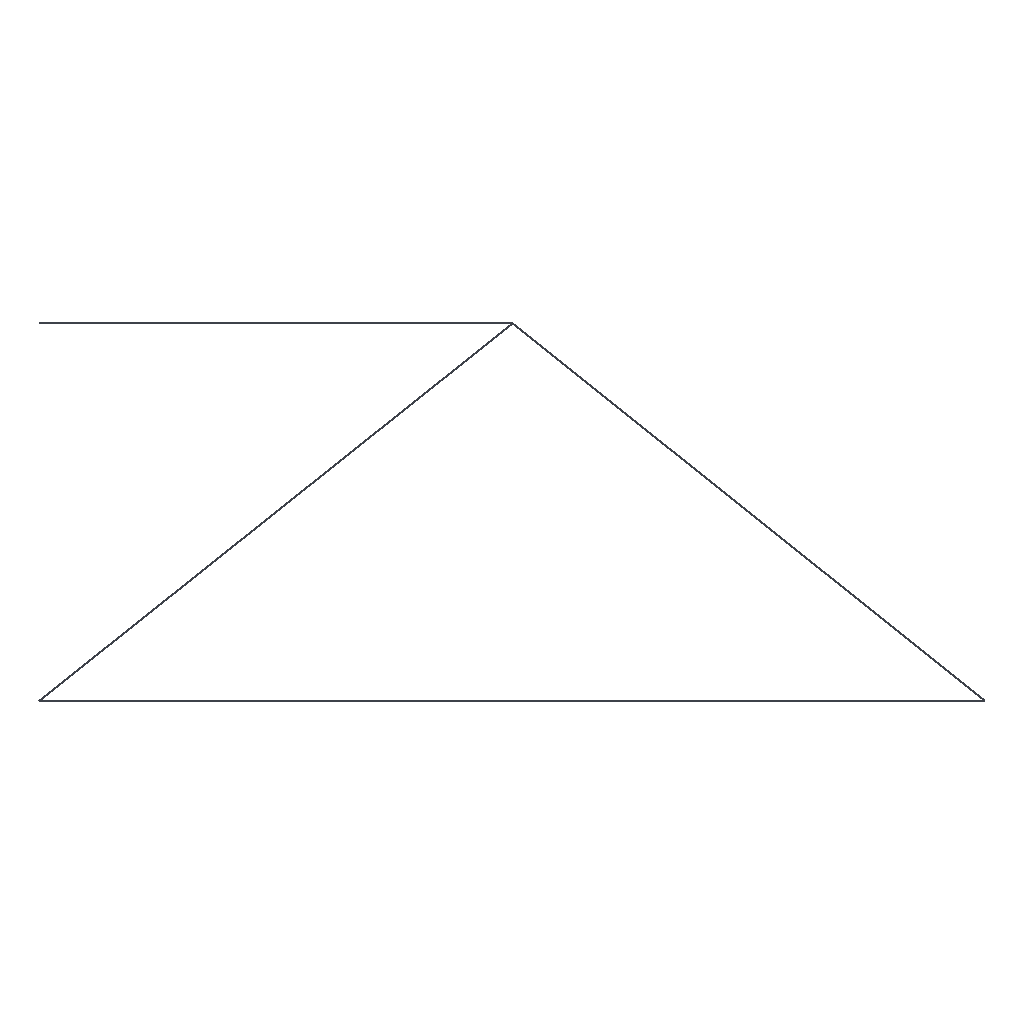Simulation study | abaqus
Set-up summary:
category,name,step,type,value,unit,region
solver,abaqus,,Abaqus/CAE 2024
units,mm-N-s-tonne (MPa),,inferred,E=295000 density=
analysis,Step-1,,static,time_period=1
mesh,nodes,,,4
mesh,elements,,,4
element_type,T2D2,,,4
material,Material-1,,E,295000
material,Material-1,,nu,0
section,Material-1,,solid section,,,_PickedSet2
load,Load-1,Step-1,concentrated force,"100 [dir=(0, -1, 0)]",,_PickedSet6
bc,BC-1,Step-1,fixed,"[dofs=x,y n=2]",,_PickedSet4
bc,BC-2,Step-1,fixed,[dofs=y],,_PickedSet5
Abaqus input file, long lists of numbers shortened:
*Heading
** Job name: deck Model name: link
** Generated by: Abaqus/CAE 2024
*Preprint, echo=NO, model=NO, history=NO, contact=NO
**
** PARTS
**
*Part, name=Part-1
*Node
      1,         100.,          80.
      2,           0.,          80.
** (2 more lines like these left out)
*Element, type=T2D2
1, 1, 2
2, 3, 1
** (2 more lines like these left out)
*Nset, nset=_PickedSet2, internal, generate
 1,  4,  1
*Elset, elset=_PickedSet2, internal, generate
 1,  4,  1
** Section: Section-1
*Solid Section, elset=_PickedSet2, material=Material-1
10.,
*End Part
**
**
** ASSEMBLY
**
*Assembly, name=Assembly
**
*Instance, name=Part-1-1, part=Part-1
*End Instance
**
*Nset, nset=_PickedSet4, internal, instance=Part-1-1
 2, 4
*Nset, nset=_PickedSet5, internal, instance=Part-1-1
 3,
*Nset, nset=_PickedSet6, internal, instance=Part-1-1
 1,
*End Assembly
**
** MATERIALS
**
*Material, name=Material-1
*Elastic
295000.,0.
** ----------------------------------------------------------------
**
** STEP: Step-1
**
*Step, name=Step-1, nlgeom=NO
*Static
1., 1., 1e-05, 1.
**
** BOUNDARY CONDITIONS
**
** Name: BC-1 Type: Displacement/Rotation
*Boundary
_PickedSet4, 1, 1
_PickedSet4, 2, 2
** Name: BC-2 Type: Displacement/Rotation
*Boundary
_PickedSet5, 2, 2
**
** LOADS
**
** Name: Load-1   Type: Concentrated force
*Cload
_PickedSet6, 2, -100.
**
** OUTPUT REQUESTS
**
*Restart, write, frequency=0
*Print, solve=NO
**
** FIELD OUTPUT: F-Output-1
**
*Output, field, variable=PRESELECT
**
** HISTORY OUTPUT: H-Output-1
**
*Output, history, variable=PRESELECT
*End Step
Results summary:
result,odb.job_status,,,JOB_STATUS_COMPLETED_SUCCESSFULLY,"consistent, unstated (Abaqus has no unit system)"
result,steps[0].procedure,Step-1,,*STATIC,"consistent, unstated (Abaqus has no unit system)"
result,steps[0].time_period,Step-1,,1,"consistent, unstated (Abaqus has no unit system)"
result,steps[0].n_frames,Step-1,,2,"consistent, unstated (Abaqus has no unit system)"
result,steps[0].last_frame.id,Step-1,,1,"consistent, unstated (Abaqus has no unit system)"
result,steps[0].last_frame.value,Step-1,,1,"consistent, unstated (Abaqus has no unit system)"
result,steps[0].last_frame.description,Step-1,,Increment      1: Step Time =    1.000,"consistent, unstated (Abaqus has no unit system)"
result,steps[0].completed,Step-1,,True,"consistent, unstated (Abaqus has no unit system)"
result,steps[0].max_U_magnitude,Step-1,,0.007736,"consistent, unstated (Abaqus has no unit system)"
result,steps[0].max_S_mises,Step-1,,9.573,"consistent, unstated (Abaqus has no unit system)"
result,steps[0].RF_sum[1],Step-1,,0,"consistent, unstated (Abaqus has no unit system)"
result,steps[0].RF_sum[2],Step-1,,100,"consistent, unstated (Abaqus has no unit system)"
result,steps[0].diagnostic.n_increments,Step-1,,1,"consistent, unstated (Abaqus has no unit system)"